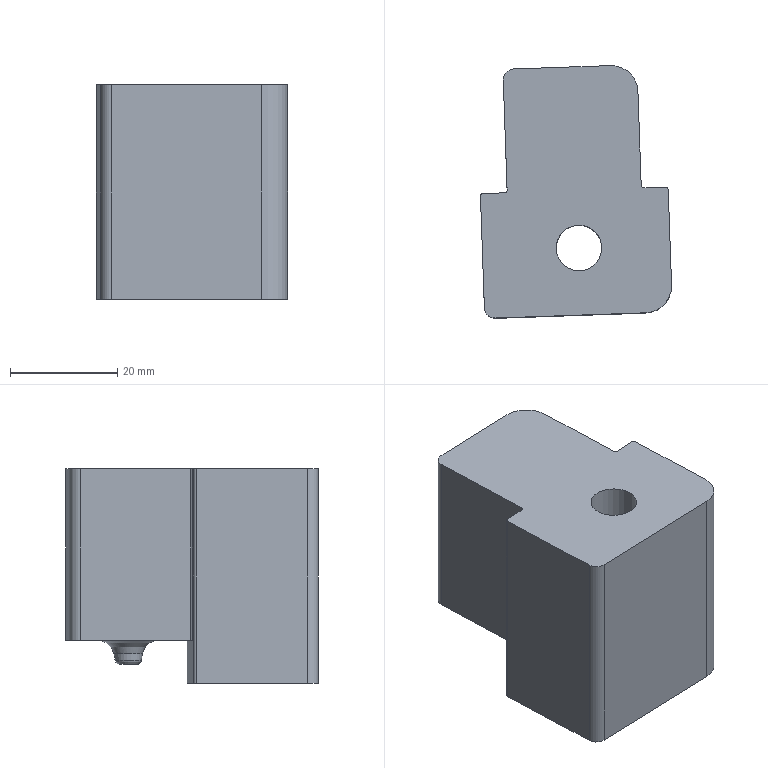Part | NX | features PS-26 2 | 1 solid | 25 faces | box 35.602 x 47.042 x 40 mm | volume 46319 mm3 | plane 12 | cylinder 10 | torus 2 | cone 1 | commonest cylinder face diameters 1 x4 4 x2 10 x2 8.506 x1 14.5 x1
STEP:
#1=CARTESIAN_POINT('',(3246.24,-821.618,900.716));
#2=VERTEX_POINT('',#1);
#3=CARTESIAN_POINT('',(3246.722,-821.101,900.716));
#4=VERTEX_POINT('',#3);
#5=CARTESIAN_POINT('',(3246.222,-821.119,900.716));
#6=DIRECTION('',(0.,0.,1.));
#7=DIRECTION('',(0.,-1.,0.));
#8=AXIS2_PLACEMENT_3D('',#5,#6,#7);
#9=CIRCLE('',#8,0.5);
#10=EDGE_CURVE('',#2,#4,#9,.T.);
#11=ORIENTED_EDGE('',*,*,#10,.F.);
#12=CARTESIAN_POINT('',(3242.242,-821.758,900.716));
#13=VERTEX_POINT('',#12);
#14=CARTESIAN_POINT('',(3256.544,-821.259,900.716));
#15=DIRECTION('',(-0.9994,-0.0349,0.));
#16=VECTOR('',#15,1000.);
#17=LINE('',#14,#16);
#18=EDGE_CURVE('',#13,#2,#17,.F.);
#19=ORIENTED_EDGE('',*,*,#18,.F.);
#20=CARTESIAN_POINT('',(3241.76,-822.275,900.716));
#21=VERTEX_POINT('',#20);
#22=CARTESIAN_POINT('',(3242.26,-822.258,900.716));
#23=DIRECTION('',(0.,0.,1.));
#24=DIRECTION('',(0.,-1.,0.));
#25=AXIS2_PLACEMENT_3D('',#22,#23,#24);
#26=CIRCLE('',#25,0.5);
#27=EDGE_CURVE('',#21,#13,#26,.F.);
#28=ORIENTED_EDGE('',*,*,#27,.F.);
#29=CARTESIAN_POINT('',(3242.484,-843.025,900.716));
#30=VERTEX_POINT('',#29);
#31=CARTESIAN_POINT('',(3239.834,-767.126,900.716));
#32=DIRECTION('',(-0.0349,0.9994,0.));
#33=VECTOR('',#32,1000.);
#34=LINE('',#31,#33);
#35=EDGE_CURVE('',#21,#30,#34,.F.);
#36=ORIENTED_EDGE('',*,*,#35,.T.);
#37=CARTESIAN_POINT('',(3244.553,-844.954,900.716));
#38=VERTEX_POINT('',#37);
#39=CARTESIAN_POINT('',(3244.483,-842.956,900.716));
#40=DIRECTION('',(0.,0.,1.));
#41=DIRECTION('',(0.,-1.,0.));
#42=AXIS2_PLACEMENT_3D('',#39,#40,#41);
#43=CIRCLE('',#42,2.);
#44=EDGE_CURVE('',#30,#38,#43,.T.);
#45=ORIENTED_EDGE('',*,*,#44,.T.);
#46=CARTESIAN_POINT('',(3272.536,-843.977,900.716));
#47=VERTEX_POINT('',#46);
#48=CARTESIAN_POINT('',(3101.644,-849.944,900.716));
#49=DIRECTION('',(-0.9994,-0.0349,0.));
#50=VECTOR('',#49,1000.);
#51=LINE('',#48,#50);
#52=EDGE_CURVE('',#47,#38,#51,.T.);
#53=ORIENTED_EDGE('',*,*,#52,.F.);
#54=CARTESIAN_POINT('',(3277.358,-838.806,900.716));
#55=VERTEX_POINT('',#54);
#56=CARTESIAN_POINT('',(3272.362,-838.98,900.716));
#57=DIRECTION('',(0.,0.,1.));
#58=DIRECTION('',(0.,-1.,0.));
#59=AXIS2_PLACEMENT_3D('',#56,#57,#58);
#60=CIRCLE('',#59,5.);
#61=EDGE_CURVE('',#47,#55,#60,.T.);
#62=ORIENTED_EDGE('',*,*,#61,.T.);
#63=CARTESIAN_POINT('',(3276.739,-821.054,900.716));
#64=VERTEX_POINT('',#63);
#65=CARTESIAN_POINT('',(3274.813,-765.904,900.716));
#66=DIRECTION('',(-0.0349,0.9994,0.));
#67=VECTOR('',#66,1000.);
#68=LINE('',#65,#67);
#69=EDGE_CURVE('',#64,#55,#68,.F.);
#70=ORIENTED_EDGE('',*,*,#69,.F.);
#71=CARTESIAN_POINT('',(3276.221,-820.572,900.716));
#72=VERTEX_POINT('',#71);
#73=CARTESIAN_POINT('',(3276.239,-821.071,900.716));
#74=DIRECTION('',(0.,0.,1.));
#75=DIRECTION('',(0.,-1.,0.));
#76=AXIS2_PLACEMENT_3D('',#73,#74,#75);
#77=CIRCLE('',#76,0.5);
#78=EDGE_CURVE('',#72,#64,#77,.F.);
#79=ORIENTED_EDGE('',*,*,#78,.F.);
#80=CARTESIAN_POINT('',(3272.224,-820.711,900.716));
#81=VERTEX_POINT('',#80);
#82=CARTESIAN_POINT('',(3256.544,-821.259,900.716));
#83=DIRECTION('',(-0.9994,-0.0349,0.));
#84=VECTOR('',#83,1000.);
#85=LINE('',#82,#84);
#86=EDGE_CURVE('',#81,#72,#85,.F.);
#87=ORIENTED_EDGE('',*,*,#86,.F.);
#88=CARTESIAN_POINT('',(3271.707,-820.229,900.716));
#89=VERTEX_POINT('',#88);
#90=CARTESIAN_POINT('',(3272.206,-820.211,900.716));
#91=DIRECTION('',(0.,0.,1.));
#92=DIRECTION('',(0.,-1.,0.));
#93=AXIS2_PLACEMENT_3D('',#90,#91,#92);
#94=CIRCLE('',#93,0.5);
#95=EDGE_CURVE('',#89,#81,#94,.T.);
#96=ORIENTED_EDGE('',*,*,#95,.F.);
#97=CARTESIAN_POINT('',(3271.096,-802.74,900.716));
#98=VERTEX_POINT('',#97);
#99=CARTESIAN_POINT('',(3269.816,-766.079,900.716));
#100=DIRECTION('',(-0.0349,0.9994,0.));
#101=VECTOR('',#100,1000.);
#102=LINE('',#99,#101);
#103=EDGE_CURVE('',#98,#89,#102,.F.);
#104=ORIENTED_EDGE('',*,*,#103,.F.);
#105=CARTESIAN_POINT('',(3265.925,-797.917,900.716));
#106=VERTEX_POINT('',#105);
#107=CARTESIAN_POINT('',(3266.099,-802.914,900.716));
#108=DIRECTION('',(0.,0.,1.));
#109=DIRECTION('',(0.,-1.,0.));
#110=AXIS2_PLACEMENT_3D('',#107,#108,#109);
#111=CIRCLE('',#110,5.);
#112=EDGE_CURVE('',#98,#106,#111,.T.);
#113=ORIENTED_EDGE('',*,*,#112,.T.);
#114=CARTESIAN_POINT('',(3247.936,-798.545,900.716));
#115=VERTEX_POINT('',#114);
#116=CARTESIAN_POINT('',(3255.742,-798.273,900.716));
#117=DIRECTION('',(-0.9994,-0.0349,0.));
#118=VECTOR('',#117,1000.);
#119=LINE('',#116,#118);
#120=EDGE_CURVE('',#106,#115,#119,.T.);
#121=ORIENTED_EDGE('',*,*,#120,.T.);
#122=CARTESIAN_POINT('',(3246.007,-800.614,900.716));
#123=VERTEX_POINT('',#122);
#124=CARTESIAN_POINT('',(3248.005,-800.544,900.716));
#125=DIRECTION('',(0.,0.,1.));
#126=DIRECTION('',(0.,-1.,0.));
#127=AXIS2_PLACEMENT_3D('',#124,#125,#126);
#128=CIRCLE('',#127,2.);
#129=EDGE_CURVE('',#115,#123,#128,.T.);
#130=ORIENTED_EDGE('',*,*,#129,.T.);
#131=CARTESIAN_POINT('',(3244.831,-766.951,900.716));
#132=DIRECTION('',(-0.0349,0.9994,0.));
#133=VECTOR('',#132,1000.);
#134=LINE('',#131,#133);
#135=EDGE_CURVE('',#123,#4,#134,.F.);
#136=ORIENTED_EDGE('',*,*,#135,.T.);
#137=EDGE_LOOP('',(#11,#19,#28,#36,#45,#53,#62,#70,#79,#87,#96,#104,#113,#121,#130,#136));
#138=FACE_BOUND('',#137,.T.);
#139=CARTESIAN_POINT('',(3260.107,-836.157,900.716));
#140=VERTEX_POINT('',#139);
#141=CARTESIAN_POINT('',(3260.107,-831.904,900.716));
#142=DIRECTION('',(0.,0.,1.));
#143=DIRECTION('',(0.,-1.,0.));
#144=AXIS2_PLACEMENT_3D('',#141,#142,#143);
#145=CIRCLE('',#144,4.253);
#146=EDGE_CURVE('',#140,#140,#145,.F.);
#147=ORIENTED_EDGE('',*,*,#146,.T.);
#148=EDGE_LOOP('',(#147));
#149=FACE_BOUND('',#148,.T.);
#150=CARTESIAN_POINT('',(3098.924,-772.046,900.716));
#151=DIRECTION('',(0.,0.,1.));
#152=DIRECTION('',(0.9976,0.06975,0.));
#153=AXIS2_PLACEMENT_3D('',#150,#151,#152);
#154=PLANE('',#153);
#155=ADVANCED_FACE('',(#138,#149),#154,.T.);
#156=CARTESIAN_POINT('',(3246.24,-821.618,868.716));
#157=VERTEX_POINT('',#156);
#158=CARTESIAN_POINT('',(3272.224,-820.711,868.716));
#159=VERTEX_POINT('',#158);
#160=CARTESIAN_POINT('',(3259.671,-821.149,868.716));
#161=DIRECTION('',(0.9994,0.0349,0.));
#162=VECTOR('',#161,1000.);
#163=LINE('',#160,#162);
#164=EDGE_CURVE('',#157,#159,#163,.T.);
#165=ORIENTED_EDGE('',*,*,#164,.F.);
#166=CARTESIAN_POINT('',(3246.722,-821.101,868.716));
#167=VERTEX_POINT('',#166);
#168=CARTESIAN_POINT('',(3246.222,-821.119,868.716));
#169=DIRECTION('',(0.,0.,1.));
#170=DIRECTION('',(-1.,0.,0.));
#171=AXIS2_PLACEMENT_3D('',#168,#169,#170);
#172=CIRCLE('',#171,0.5);
#173=EDGE_CURVE('',#167,#157,#172,.F.);
#174=ORIENTED_EDGE('',*,*,#173,.F.);
#175=CARTESIAN_POINT('',(3246.007,-800.614,868.716));
#176=VERTEX_POINT('',#175);
#177=CARTESIAN_POINT('',(3246.334,-809.99,868.716));
#178=DIRECTION('',(0.0349,-0.9994,0.));
#179=VECTOR('',#178,1000.);
#180=LINE('',#177,#179);
#181=EDGE_CURVE('',#176,#167,#180,.T.);
#182=ORIENTED_EDGE('',*,*,#181,.F.);
#183=CARTESIAN_POINT('',(3247.936,-798.545,868.716));
#184=VERTEX_POINT('',#183);
#185=CARTESIAN_POINT('',(3248.005,-800.544,868.716));
#186=DIRECTION('',(0.,0.,1.));
#187=DIRECTION('',(-1.,0.,0.));
#188=AXIS2_PLACEMENT_3D('',#185,#186,#187);
#189=CIRCLE('',#188,2.);
#190=EDGE_CURVE('',#176,#184,#189,.F.);
#191=ORIENTED_EDGE('',*,*,#190,.T.);
#192=CARTESIAN_POINT('',(3265.925,-797.917,868.716));
#193=VERTEX_POINT('',#192);
#194=CARTESIAN_POINT('',(3258.868,-798.163,868.716));
#195=DIRECTION('',(-0.9994,-0.0349,0.));
#196=VECTOR('',#195,1000.);
#197=LINE('',#194,#196);
#198=EDGE_CURVE('',#184,#193,#197,.F.);
#199=ORIENTED_EDGE('',*,*,#198,.T.);
#200=CARTESIAN_POINT('',(3271.096,-802.74,868.716));
#201=VERTEX_POINT('',#200);
#202=CARTESIAN_POINT('',(3266.099,-802.914,868.716));
#203=DIRECTION('',(0.,0.,1.));
#204=DIRECTION('',(-1.,0.,0.));
#205=AXIS2_PLACEMENT_3D('',#202,#203,#204);
#206=CIRCLE('',#205,5.);
#207=EDGE_CURVE('',#193,#201,#206,.F.);
#208=ORIENTED_EDGE('',*,*,#207,.T.);
#209=CARTESIAN_POINT('',(3271.707,-820.229,868.716));
#210=VERTEX_POINT('',#209);
#211=CARTESIAN_POINT('',(3271.319,-809.117,868.716));
#212=DIRECTION('',(0.0349,-0.9994,0.));
#213=VECTOR('',#212,1000.);
#214=LINE('',#211,#213);
#215=EDGE_CURVE('',#201,#210,#214,.T.);
#216=ORIENTED_EDGE('',*,*,#215,.T.);
#217=CARTESIAN_POINT('',(3272.206,-820.211,868.716));
#218=DIRECTION('',(0.,0.,1.));
#219=DIRECTION('',(-1.,0.,0.));
#220=AXIS2_PLACEMENT_3D('',#217,#218,#219);
#221=CIRCLE('',#220,0.5);
#222=EDGE_CURVE('',#159,#210,#221,.F.);
#223=ORIENTED_EDGE('',*,*,#222,.F.);
#224=EDGE_LOOP('',(#165,#174,#182,#191,#199,#208,#216,#223));
#225=FACE_BOUND('',#224,.T.);
#226=CARTESIAN_POINT('',(3253.659,-809.93,868.716));
#227=VERTEX_POINT('',#226);
#228=CARTESIAN_POINT('',(3259.266,-809.538,868.716));
#229=DIRECTION('',(0.,0.,1.));
#230=DIRECTION('',(-0.9976,-0.06975,0.));
#231=AXIS2_PLACEMENT_3D('',#228,#229,#230);
#232=CIRCLE('',#231,5.62);
#233=EDGE_CURVE('',#227,#227,#232,.T.);
#234=ORIENTED_EDGE('',*,*,#233,.T.);
#235=EDGE_LOOP('',(#234));
#236=FACE_BOUND('',#235,.T.);
#237=CARTESIAN_POINT('',(3259.266,-809.538,868.716));
#238=DIRECTION('',(0.,0.,-1.));
#239=DIRECTION('',(-0.0349,0.9994,0.));
#240=AXIS2_PLACEMENT_3D('',#237,#238,#239);
#241=PLANE('',#240);
#242=ADVANCED_FACE('',(#225,#236),#241,.T.);
#243=ORIENTED_EDGE('',*,*,#129,.F.);
#244=CARTESIAN_POINT('',(3247.936,-798.545,884.716));
#245=DIRECTION('',(0.,0.,1.));
#246=VECTOR('',#245,1000.);
#247=LINE('',#244,#246);
#248=EDGE_CURVE('',#115,#184,#247,.F.);
#249=ORIENTED_EDGE('',*,*,#248,.T.);
#250=ORIENTED_EDGE('',*,*,#190,.F.);
#251=CARTESIAN_POINT('',(3246.007,-800.614,890.716));
#252=DIRECTION('',(0.,0.,1.));
#253=VECTOR('',#252,1000.);
#254=LINE('',#251,#253);
#255=EDGE_CURVE('',#123,#176,#254,.F.);
#256=ORIENTED_EDGE('',*,*,#255,.F.);
#257=EDGE_LOOP('',(#243,#249,#250,#256));
#258=FACE_BOUND('',#257,.T.);
#259=CARTESIAN_POINT('',(3248.005,-800.544,890.716));
#260=DIRECTION('',(0.,0.,1.));
#261=DIRECTION('',(1.,0.,0.));
#262=AXIS2_PLACEMENT_3D('',#259,#260,#261);
#263=CYLINDRICAL_SURFACE('',#262,2.);
#264=ADVANCED_FACE('',(#258),#263,.T.);
#265=ORIENTED_EDGE('',*,*,#207,.F.);
#266=CARTESIAN_POINT('',(3265.925,-797.917,884.716));
#267=DIRECTION('',(0.,0.,-1.));
#268=VECTOR('',#267,1000.);
#269=LINE('',#266,#268);
#270=EDGE_CURVE('',#193,#106,#269,.F.);
#271=ORIENTED_EDGE('',*,*,#270,.T.);
#272=ORIENTED_EDGE('',*,*,#112,.F.);
#273=CARTESIAN_POINT('',(3271.096,-802.74,935.716));
#274=DIRECTION('',(0.,0.,1.));
#275=VECTOR('',#274,1000.);
#276=LINE('',#273,#275);
#277=EDGE_CURVE('',#201,#98,#276,.T.);
#278=ORIENTED_EDGE('',*,*,#277,.F.);
#279=EDGE_LOOP('',(#265,#271,#272,#278));
#280=FACE_BOUND('',#279,.T.);
#281=CARTESIAN_POINT('',(3266.099,-802.914,935.716));
#282=DIRECTION('',(0.,0.,-1.));
#283=DIRECTION('',(-1.,0.,0.));
#284=AXIS2_PLACEMENT_3D('',#281,#282,#283);
#285=CYLINDRICAL_SURFACE('',#284,5.);
#286=ADVANCED_FACE('',(#280),#285,.T.);
#287=ORIENTED_EDGE('',*,*,#215,.F.);
#288=ORIENTED_EDGE('',*,*,#277,.T.);
#289=ORIENTED_EDGE('',*,*,#103,.T.);
#290=CARTESIAN_POINT('',(3271.707,-820.229,862.716));
#291=DIRECTION('',(0.,0.,1.));
#292=VECTOR('',#291,1000.);
#293=LINE('',#290,#292);
#294=EDGE_CURVE('',#210,#89,#293,.T.);
#295=ORIENTED_EDGE('',*,*,#294,.F.);
#296=EDGE_LOOP('',(#287,#288,#289,#295));
#297=FACE_BOUND('',#296,.T.);
#298=CARTESIAN_POINT('',(3271.54,-815.453,862.716));
#299=DIRECTION('',(0.9994,0.0349,0.));
#300=DIRECTION('',(-0.0349,0.9994,0.));
#301=AXIS2_PLACEMENT_3D('',#298,#299,#300);
#302=PLANE('',#301);
#303=ADVANCED_FACE('',(#297),#302,.T.);
#304=ORIENTED_EDGE('',*,*,#135,.F.);
#305=ORIENTED_EDGE('',*,*,#255,.T.);
#306=ORIENTED_EDGE('',*,*,#181,.T.);
#307=CARTESIAN_POINT('',(3246.722,-821.101,868.716));
#308=DIRECTION('',(0.,0.,-1.));
#309=VECTOR('',#308,1000.);
#310=LINE('',#307,#309);
#311=EDGE_CURVE('',#4,#167,#310,.T.);
#312=ORIENTED_EDGE('',*,*,#311,.F.);
#313=EDGE_LOOP('',(#304,#305,#306,#312));
#314=FACE_BOUND('',#313,.T.);
#315=CARTESIAN_POINT('',(3246.52,-815.326,890.716));
#316=DIRECTION('',(0.9994,0.0349,0.));
#317=DIRECTION('',(-0.0349,0.9994,0.));
#318=AXIS2_PLACEMENT_3D('',#315,#316,#317);
#319=PLANE('',#318);
#320=ADVANCED_FACE('',(#314),#319,.F.);
#321=CARTESIAN_POINT('',(3259.452,-812.197,866.237));
#322=VERTEX_POINT('',#321);
#323=CARTESIAN_POINT('',(3259.266,-809.538,866.237));
#324=DIRECTION('',(0.,0.,1.));
#325=DIRECTION('',(0.06975,-0.9976,0.));
#326=AXIS2_PLACEMENT_3D('',#323,#324,#325);
#327=CIRCLE('',#326,2.666);
#328=EDGE_CURVE('',#322,#322,#327,.T.);
#329=ORIENTED_EDGE('',*,*,#328,.T.);
#330=EDGE_LOOP('',(#329));
#331=FACE_BOUND('',#330,.T.);
#332=ORIENTED_EDGE('',*,*,#233,.F.);
#333=EDGE_LOOP('',(#332));
#334=FACE_BOUND('',#333,.T.);
#335=CARTESIAN_POINT('',(3259.266,-809.538,865.716));
#336=DIRECTION('',(0.,0.,-1.));
#337=DIRECTION('',(0.06975,-0.9976,0.));
#338=AXIS2_PLACEMENT_3D('',#335,#336,#337);
#339=TOROIDAL_SURFACE('',#338,5.62,3.);
#340=ADVANCED_FACE('',(#331,#334),#339,.F.);
#341=CARTESIAN_POINT('',(3259.437,-811.987,865.043));
#342=VERTEX_POINT('',#341);
#343=CARTESIAN_POINT('',(3259.266,-809.538,865.043));
#344=DIRECTION('',(0.,0.,1.));
#345=DIRECTION('',(0.06975,-0.9976,0.));
#346=AXIS2_PLACEMENT_3D('',#343,#344,#345);
#347=CIRCLE('',#346,2.455);
#348=EDGE_CURVE('',#342,#342,#347,.T.);
#349=ORIENTED_EDGE('',*,*,#348,.T.);
#350=EDGE_LOOP('',(#349));
#351=FACE_BOUND('',#350,.T.);
#352=ORIENTED_EDGE('',*,*,#328,.F.);
#353=EDGE_LOOP('',(#352));
#354=FACE_BOUND('',#353,.T.);
#355=CARTESIAN_POINT('',(3259.266,-809.538,866.237));
#356=DIRECTION('',(0.,0.,1.));
#357=DIRECTION('',(-0.06975,0.9976,0.));
#358=AXIS2_PLACEMENT_3D('',#355,#356,#357);
#359=CONICAL_SURFACE('',#358,2.666,0.1745);
#360=ADVANCED_FACE('',(#351,#354),#359,.T.);
#361=CARTESIAN_POINT('',(3260.962,-809.419,864.243));
#362=VERTEX_POINT('',#361);
#363=CARTESIAN_POINT('',(3259.266,-809.538,864.243));
#364=DIRECTION('',(0.,0.,1.));
#365=DIRECTION('',(0.9976,0.06975,0.));
#366=AXIS2_PLACEMENT_3D('',#363,#364,#365);
#367=CIRCLE('',#366,1.7);
#368=EDGE_CURVE('',#362,#362,#367,.T.);
#369=ORIENTED_EDGE('',*,*,#368,.T.);
#370=EDGE_LOOP('',(#369));
#371=FACE_BOUND('',#370,.T.);
#372=ORIENTED_EDGE('',*,*,#348,.F.);
#373=EDGE_LOOP('',(#372));
#374=FACE_BOUND('',#373,.T.);
#375=CARTESIAN_POINT('',(3259.266,-809.538,865.216));
#376=DIRECTION('',(0.,0.,-1.));
#377=DIRECTION('',(0.06975,-0.9976,0.));
#378=AXIS2_PLACEMENT_3D('',#375,#376,#377);
#379=TOROIDAL_SURFACE('',#378,1.47,1.);
#380=ADVANCED_FACE('',(#371,#374),#379,.T.);
#381=ORIENTED_EDGE('',*,*,#368,.F.);
#382=EDGE_LOOP('',(#381));
#383=FACE_BOUND('',#382,.T.);
#384=CARTESIAN_POINT('',(3259.266,-809.538,864.243));
#385=DIRECTION('',(0.,0.,1.));
#386=DIRECTION('',(0.9976,0.06975,0.));
#387=AXIS2_PLACEMENT_3D('',#384,#385,#386);
#388=PLANE('',#387);
#389=ADVANCED_FACE('',(#383),#388,.F.);
#390=ORIENTED_EDGE('',*,*,#222,.T.);
#391=ORIENTED_EDGE('',*,*,#294,.T.);
#392=ORIENTED_EDGE('',*,*,#95,.T.);
#393=CARTESIAN_POINT('',(3272.224,-820.711,863.216));
#394=DIRECTION('',(0.,0.,1.));
#395=VECTOR('',#394,1000.);
#396=LINE('',#393,#395);
#397=EDGE_CURVE('',#81,#159,#396,.F.);
#398=ORIENTED_EDGE('',*,*,#397,.T.);
#399=EDGE_LOOP('',(#390,#391,#392,#398));
#400=FACE_BOUND('',#399,.T.);
#401=CARTESIAN_POINT('',(3272.206,-820.211,862.716));
#402=DIRECTION('',(0.,0.,1.));
#403=DIRECTION('',(1.,0.,0.));
#404=AXIS2_PLACEMENT_3D('',#401,#402,#403);
#405=CYLINDRICAL_SURFACE('',#404,0.5);
#406=ADVANCED_FACE('',(#400),#405,.F.);
#407=ORIENTED_EDGE('',*,*,#10,.T.);
#408=ORIENTED_EDGE('',*,*,#311,.T.);
#409=ORIENTED_EDGE('',*,*,#173,.T.);
#410=CARTESIAN_POINT('',(3246.24,-821.618,890.716));
#411=DIRECTION('',(0.,0.,-1.));
#412=VECTOR('',#411,1000.);
#413=LINE('',#410,#412);
#414=EDGE_CURVE('',#157,#2,#413,.F.);
#415=ORIENTED_EDGE('',*,*,#414,.T.);
#416=EDGE_LOOP('',(#407,#408,#409,#415));
#417=FACE_BOUND('',#416,.T.);
#418=CARTESIAN_POINT('',(3246.222,-821.119,890.716));
#419=DIRECTION('',(0.,0.,1.));
#420=DIRECTION('',(1.,0.,0.));
#421=AXIS2_PLACEMENT_3D('',#418,#419,#420);
#422=CYLINDRICAL_SURFACE('',#421,0.5);
#423=ADVANCED_FACE('',(#417),#422,.F.);
#424=ORIENTED_EDGE('',*,*,#248,.F.);
#425=ORIENTED_EDGE('',*,*,#120,.F.);
#426=ORIENTED_EDGE('',*,*,#270,.F.);
#427=ORIENTED_EDGE('',*,*,#198,.F.);
#428=EDGE_LOOP('',(#424,#425,#426,#427));
#429=FACE_BOUND('',#428,.T.);
#430=CARTESIAN_POINT('',(3255.742,-798.273,863.216));
#431=DIRECTION('',(0.0349,-0.9994,0.));
#432=DIRECTION('',(-0.9994,-0.0349,0.));
#433=AXIS2_PLACEMENT_3D('',#430,#431,#432);
#434=PLANE('',#433);
#435=ADVANCED_FACE('',(#429),#434,.F.);
#436=CARTESIAN_POINT('',(3264.35,-831.607,879.716));
#437=VERTEX_POINT('',#436);
#438=CARTESIAN_POINT('',(3260.107,-831.904,879.716));
#439=DIRECTION('',(0.,0.,1.));
#440=DIRECTION('',(0.9976,0.06975,0.));
#441=AXIS2_PLACEMENT_3D('',#438,#439,#440);
#442=CIRCLE('',#441,4.253);
#443=EDGE_CURVE('',#437,#437,#442,.T.);
#444=ORIENTED_EDGE('',*,*,#443,.T.);
#445=EDGE_LOOP('',(#444));
#446=FACE_BOUND('',#445,.T.);
#447=CARTESIAN_POINT('',(3267.339,-831.398,879.716));
#448=VERTEX_POINT('',#447);
#449=CARTESIAN_POINT('',(3260.107,-831.904,879.716));
#450=DIRECTION('',(0.,0.,-1.));
#451=DIRECTION('',(0.9976,0.06975,0.));
#452=AXIS2_PLACEMENT_3D('',#449,#450,#451);
#453=CIRCLE('',#452,7.25);
#454=EDGE_CURVE('',#448,#448,#453,.F.);
#455=ORIENTED_EDGE('',*,*,#454,.F.);
#456=EDGE_LOOP('',(#455));
#457=FACE_BOUND('',#456,.T.);
#458=CARTESIAN_POINT('',(3260.107,-831.904,879.716));
#459=DIRECTION('',(0.,0.,1.));
#460=DIRECTION('',(0.9976,0.06975,0.));
#461=AXIS2_PLACEMENT_3D('',#458,#459,#460);
#462=PLANE('',#461);
#463=ADVANCED_FACE('',(#446,#457),#462,.F.);
#464=ORIENTED_EDGE('',*,*,#443,.F.);
#465=EDGE_LOOP('',(#464));
#466=FACE_BOUND('',#465,.T.);
#467=ORIENTED_EDGE('',*,*,#146,.F.);
#468=EDGE_LOOP('',(#467));
#469=FACE_BOUND('',#468,.T.);
#470=CARTESIAN_POINT('',(3260.107,-831.904,868.716));
#471=DIRECTION('',(0.,0.,1.));
#472=DIRECTION('',(0.9976,0.06975,0.));
#473=AXIS2_PLACEMENT_3D('',#470,#471,#472);
#474=CYLINDRICAL_SURFACE('',#473,4.253);
#475=ADVANCED_FACE('',(#466,#469),#474,.F.);
#476=CARTESIAN_POINT('',(3242.242,-821.758,860.716));
#477=VERTEX_POINT('',#476);
#478=CARTESIAN_POINT('',(3241.76,-822.275,860.716));
#479=VERTEX_POINT('',#478);
#480=CARTESIAN_POINT('',(3242.26,-822.258,860.716));
#481=DIRECTION('',(0.,0.,1.));
#482=DIRECTION('',(1.,0.,0.));
#483=AXIS2_PLACEMENT_3D('',#480,#481,#482);
#484=CIRCLE('',#483,0.5);
#485=EDGE_CURVE('',#477,#479,#484,.T.);
#486=ORIENTED_EDGE('',*,*,#485,.T.);
#487=CARTESIAN_POINT('',(3241.76,-822.275,890.716));
#488=DIRECTION('',(0.,0.,1.));
#489=VECTOR('',#488,1000.);
#490=LINE('',#487,#489);
#491=EDGE_CURVE('',#479,#21,#490,.T.);
#492=ORIENTED_EDGE('',*,*,#491,.T.);
#493=ORIENTED_EDGE('',*,*,#27,.T.);
#494=CARTESIAN_POINT('',(3242.242,-821.758,863.216));
#495=DIRECTION('',(0.,0.,1.));
#496=VECTOR('',#495,1000.);
#497=LINE('',#494,#496);
#498=EDGE_CURVE('',#13,#477,#497,.F.);
#499=ORIENTED_EDGE('',*,*,#498,.T.);
#500=EDGE_LOOP('',(#486,#492,#493,#499));
#501=FACE_BOUND('',#500,.T.);
#502=CARTESIAN_POINT('',(3242.26,-822.258,890.716));
#503=DIRECTION('',(0.,0.,1.));
#504=DIRECTION('',(1.,0.,0.));
#505=AXIS2_PLACEMENT_3D('',#502,#503,#504);
#506=CYLINDRICAL_SURFACE('',#505,0.5);
#507=ADVANCED_FACE('',(#501),#506,.T.);
#508=CARTESIAN_POINT('',(3242.484,-843.025,860.716));
#509=VERTEX_POINT('',#508);
#510=CARTESIAN_POINT('',(3247.475,-985.945,860.716));
#511=DIRECTION('',(-0.0349,0.9994,0.));
#512=VECTOR('',#511,1000.);
#513=LINE('',#510,#512);
#514=EDGE_CURVE('',#479,#509,#513,.F.);
#515=ORIENTED_EDGE('',*,*,#514,.T.);
#516=CARTESIAN_POINT('',(3242.484,-843.025,890.716));
#517=DIRECTION('',(0.,0.,1.));
#518=VECTOR('',#517,1000.);
#519=LINE('',#516,#518);
#520=EDGE_CURVE('',#509,#30,#519,.T.);
#521=ORIENTED_EDGE('',*,*,#520,.T.);
#522=ORIENTED_EDGE('',*,*,#35,.F.);
#523=ORIENTED_EDGE('',*,*,#491,.F.);
#524=EDGE_LOOP('',(#515,#521,#522,#523));
#525=FACE_BOUND('',#524,.T.);
#526=CARTESIAN_POINT('',(3241.523,-815.501,890.716));
#527=DIRECTION('',(0.9994,0.0349,0.));
#528=DIRECTION('',(-0.0349,0.9994,0.));
#529=AXIS2_PLACEMENT_3D('',#526,#527,#528);
#530=PLANE('',#529);
#531=ADVANCED_FACE('',(#525),#530,.F.);
#532=ORIENTED_EDGE('',*,*,#44,.F.);
#533=ORIENTED_EDGE('',*,*,#520,.F.);
#534=CARTESIAN_POINT('',(3244.553,-844.954,860.716));
#535=VERTEX_POINT('',#534);
#536=CARTESIAN_POINT('',(3244.483,-842.956,860.716));
#537=DIRECTION('',(0.,0.,1.));
#538=DIRECTION('',(1.,0.,0.));
#539=AXIS2_PLACEMENT_3D('',#536,#537,#538);
#540=CIRCLE('',#539,2.);
#541=EDGE_CURVE('',#535,#509,#540,.F.);
#542=ORIENTED_EDGE('',*,*,#541,.F.);
#543=CARTESIAN_POINT('',(3244.553,-844.954,860.716));
#544=DIRECTION('',(0.,0.,-1.));
#545=VECTOR('',#544,1000.);
#546=LINE('',#543,#545);
#547=EDGE_CURVE('',#38,#535,#546,.T.);
#548=ORIENTED_EDGE('',*,*,#547,.F.);
#549=EDGE_LOOP('',(#532,#533,#542,#548));
#550=FACE_BOUND('',#549,.T.);
#551=CARTESIAN_POINT('',(3244.483,-842.956,935.716));
#552=DIRECTION('',(0.,0.,-1.));
#553=DIRECTION('',(-0.9976,-0.06975,0.));
#554=AXIS2_PLACEMENT_3D('',#551,#552,#553);
#555=CYLINDRICAL_SURFACE('',#554,2.);
#556=ADVANCED_FACE('',(#550),#555,.T.);
#557=CARTESIAN_POINT('',(3272.536,-843.977,860.716));
#558=VERTEX_POINT('',#557);
#559=CARTESIAN_POINT('',(3231.561,-845.408,860.716));
#560=DIRECTION('',(0.9994,0.0349,0.));
#561=VECTOR('',#560,1000.);
#562=LINE('',#559,#561);
#563=EDGE_CURVE('',#535,#558,#562,.T.);
#564=ORIENTED_EDGE('',*,*,#563,.T.);
#565=CARTESIAN_POINT('',(3272.536,-843.977,935.716));
#566=DIRECTION('',(0.,0.,-1.));
#567=VECTOR('',#566,1000.);
#568=LINE('',#565,#567);
#569=EDGE_CURVE('',#558,#47,#568,.F.);
#570=ORIENTED_EDGE('',*,*,#569,.T.);
#571=ORIENTED_EDGE('',*,*,#52,.T.);
#572=ORIENTED_EDGE('',*,*,#547,.T.);
#573=EDGE_LOOP('',(#564,#570,#571,#572));
#574=FACE_BOUND('',#573,.T.);
#575=CARTESIAN_POINT('',(3231.561,-845.408,935.716));
#576=DIRECTION('',(-0.0349,0.9994,0.));
#577=DIRECTION('',(-0.9994,-0.0349,0.));
#578=AXIS2_PLACEMENT_3D('',#575,#576,#577);
#579=PLANE('',#578);
#580=ADVANCED_FACE('',(#574),#579,.F.);
#581=ORIENTED_EDGE('',*,*,#61,.F.);
#582=ORIENTED_EDGE('',*,*,#569,.F.);
#583=CARTESIAN_POINT('',(3277.358,-838.806,860.716));
#584=VERTEX_POINT('',#583);
#585=CARTESIAN_POINT('',(3272.362,-838.98,860.716));
#586=DIRECTION('',(0.,0.,1.));
#587=DIRECTION('',(1.,0.,0.));
#588=AXIS2_PLACEMENT_3D('',#585,#586,#587);
#589=CIRCLE('',#588,5.);
#590=EDGE_CURVE('',#584,#558,#589,.F.);
#591=ORIENTED_EDGE('',*,*,#590,.F.);
#592=CARTESIAN_POINT('',(3277.358,-838.806,862.716));
#593=DIRECTION('',(0.,0.,1.));
#594=VECTOR('',#593,1000.);
#595=LINE('',#592,#594);
#596=EDGE_CURVE('',#55,#584,#595,.F.);
#597=ORIENTED_EDGE('',*,*,#596,.F.);
#598=EDGE_LOOP('',(#581,#582,#591,#597));
#599=FACE_BOUND('',#598,.T.);
#600=CARTESIAN_POINT('',(3272.362,-838.98,862.716));
#601=DIRECTION('',(0.,0.,1.));
#602=DIRECTION('',(0.9976,0.06975,0.));
#603=AXIS2_PLACEMENT_3D('',#600,#601,#602);
#604=CYLINDRICAL_SURFACE('',#603,5.);
#605=ADVANCED_FACE('',(#599),#604,.T.);
#606=ORIENTED_EDGE('',*,*,#69,.T.);
#607=ORIENTED_EDGE('',*,*,#596,.T.);
#608=CARTESIAN_POINT('',(3276.739,-821.054,860.716));
#609=VERTEX_POINT('',#608);
#610=CARTESIAN_POINT('',(3282.453,-984.724,860.716));
#611=DIRECTION('',(-0.0349,0.9994,0.));
#612=VECTOR('',#611,1000.);
#613=LINE('',#610,#612);
#614=EDGE_CURVE('',#609,#584,#613,.F.);
#615=ORIENTED_EDGE('',*,*,#614,.F.);
#616=CARTESIAN_POINT('',(3276.739,-821.054,868.716));
#617=DIRECTION('',(0.,0.,-1.));
#618=VECTOR('',#617,1000.);
#619=LINE('',#616,#618);
#620=EDGE_CURVE('',#64,#609,#619,.T.);
#621=ORIENTED_EDGE('',*,*,#620,.F.);
#622=EDGE_LOOP('',(#606,#607,#615,#621));
#623=FACE_BOUND('',#622,.T.);
#624=CARTESIAN_POINT('',(3276.537,-815.279,862.716));
#625=DIRECTION('',(0.9994,0.0349,0.));
#626=DIRECTION('',(-0.0349,0.9994,0.));
#627=AXIS2_PLACEMENT_3D('',#624,#625,#626);
#628=PLANE('',#627);
#629=ADVANCED_FACE('',(#623),#628,.T.);
#630=ORIENTED_EDGE('',*,*,#78,.T.);
#631=ORIENTED_EDGE('',*,*,#620,.T.);
#632=CARTESIAN_POINT('',(3276.221,-820.572,860.716));
#633=VERTEX_POINT('',#632);
#634=CARTESIAN_POINT('',(3276.239,-821.071,860.716));
#635=DIRECTION('',(0.,0.,1.));
#636=DIRECTION('',(1.,0.,0.));
#637=AXIS2_PLACEMENT_3D('',#634,#635,#636);
#638=CIRCLE('',#637,0.5);
#639=EDGE_CURVE('',#609,#633,#638,.T.);
#640=ORIENTED_EDGE('',*,*,#639,.T.);
#641=CARTESIAN_POINT('',(3276.221,-820.572,890.716));
#642=DIRECTION('',(0.,0.,-1.));
#643=VECTOR('',#642,1000.);
#644=LINE('',#641,#643);
#645=EDGE_CURVE('',#633,#72,#644,.F.);
#646=ORIENTED_EDGE('',*,*,#645,.T.);
#647=EDGE_LOOP('',(#630,#631,#640,#646));
#648=FACE_BOUND('',#647,.T.);
#649=CARTESIAN_POINT('',(3276.239,-821.071,862.716));
#650=DIRECTION('',(0.,0.,1.));
#651=DIRECTION('',(1.,0.,0.));
#652=AXIS2_PLACEMENT_3D('',#649,#650,#651);
#653=CYLINDRICAL_SURFACE('',#652,0.5);
#654=ADVANCED_FACE('',(#648),#653,.T.);
#655=ORIENTED_EDGE('',*,*,#454,.T.);
#656=EDGE_LOOP('',(#655));
#657=FACE_BOUND('',#656,.T.);
#658=CARTESIAN_POINT('',(3267.357,-831.904,860.716));
#659=VERTEX_POINT('',#658);
#660=CARTESIAN_POINT('',(3260.107,-831.904,860.716));
#661=DIRECTION('',(0.,0.,1.));
#662=DIRECTION('',(1.,0.,0.));
#663=AXIS2_PLACEMENT_3D('',#660,#661,#662);
#664=CIRCLE('',#663,7.25);
#665=EDGE_CURVE('',#659,#659,#664,.T.);
#666=ORIENTED_EDGE('',*,*,#665,.F.);
#667=EDGE_LOOP('',(#666));
#668=FACE_BOUND('',#667,.T.);
#669=CARTESIAN_POINT('',(3260.107,-831.904,868.716));
#670=DIRECTION('',(0.,0.,1.));
#671=DIRECTION('',(0.9976,0.06975,0.));
#672=AXIS2_PLACEMENT_3D('',#669,#670,#671);
#673=CYLINDRICAL_SURFACE('',#672,7.25);
#674=ADVANCED_FACE('',(#657,#668),#673,.F.);
#675=ORIENTED_EDGE('',*,*,#665,.T.);
#676=EDGE_LOOP('',(#675));
#677=FACE_BOUND('',#676,.T.);
#678=ORIENTED_EDGE('',*,*,#485,.F.);
#679=CARTESIAN_POINT('',(3256.544,-821.259,860.716));
#680=DIRECTION('',(-0.9994,-0.0349,0.));
#681=VECTOR('',#680,1000.);
#682=LINE('',#679,#681);
#683=EDGE_CURVE('',#477,#633,#682,.F.);
#684=ORIENTED_EDGE('',*,*,#683,.T.);
#685=ORIENTED_EDGE('',*,*,#639,.F.);
#686=ORIENTED_EDGE('',*,*,#614,.T.);
#687=ORIENTED_EDGE('',*,*,#590,.T.);
#688=ORIENTED_EDGE('',*,*,#563,.F.);
#689=ORIENTED_EDGE('',*,*,#541,.T.);
#690=ORIENTED_EDGE('',*,*,#514,.F.);
#691=EDGE_LOOP('',(#678,#684,#685,#686,#687,#688,#689,#690));
#692=FACE_BOUND('',#691,.T.);
#693=CARTESIAN_POINT('',(2870.094,-999.122,860.716));
#694=DIRECTION('',(0.,0.,1.));
#695=DIRECTION('',(0.,1.,0.));
#696=AXIS2_PLACEMENT_3D('',#693,#694,#695);
#697=PLANE('',#696);
#698=ADVANCED_FACE('',(#677,#692),#697,.F.);
#699=ORIENTED_EDGE('',*,*,#397,.F.);
#700=ORIENTED_EDGE('',*,*,#86,.T.);
#701=ORIENTED_EDGE('',*,*,#645,.F.);
#702=ORIENTED_EDGE('',*,*,#683,.F.);
#703=ORIENTED_EDGE('',*,*,#498,.F.);
#704=ORIENTED_EDGE('',*,*,#18,.T.);
#705=ORIENTED_EDGE('',*,*,#414,.F.);
#706=ORIENTED_EDGE('',*,*,#164,.T.);
#707=EDGE_LOOP('',(#699,#700,#701,#702,#703,#704,#705,#706));
#708=FACE_BOUND('',#707,.T.);
#709=CARTESIAN_POINT('',(3256.544,-821.259,863.216));
#710=DIRECTION('',(0.0349,-0.9994,0.));
#711=DIRECTION('',(-0.9994,-0.0349,0.));
#712=AXIS2_PLACEMENT_3D('',#709,#710,#711);
#713=PLANE('',#712);
#714=ADVANCED_FACE('',(#708),#713,.F.);
#715=CLOSED_SHELL('',(#155,#242,#264,#286,#303,#320,#340,#360,#380,#389,#406,#423,#435,#463,#475,#507,#531,#556,#580,#605,#629,#654,#674,#698,#714));
#716=MANIFOLD_SOLID_BREP('',#715);
#717=(LENGTH_UNIT()NAMED_UNIT(*)SI_UNIT(.MILLI.,.METRE.));
#718=UNCERTAINTY_MEASURE_WITH_UNIT(LENGTH_MEASURE(0.00001),#717,'','');
#719=(NAMED_UNIT(*)PLANE_ANGLE_UNIT()SI_UNIT($,.RADIAN.));
#720=(NAMED_UNIT(*)SI_UNIT($,.STERADIAN.)SOLID_ANGLE_UNIT());
#721=(GEOMETRIC_REPRESENTATION_CONTEXT(3)GLOBAL_UNCERTAINTY_ASSIGNED_CONTEXT((#718))GLOBAL_UNIT_ASSIGNED_CONTEXT((#717,#719,#720))REPRESENTATION_CONTEXT('',''));
#722=ADVANCED_BREP_SHAPE_REPRESENTATION('',(#716),#721);